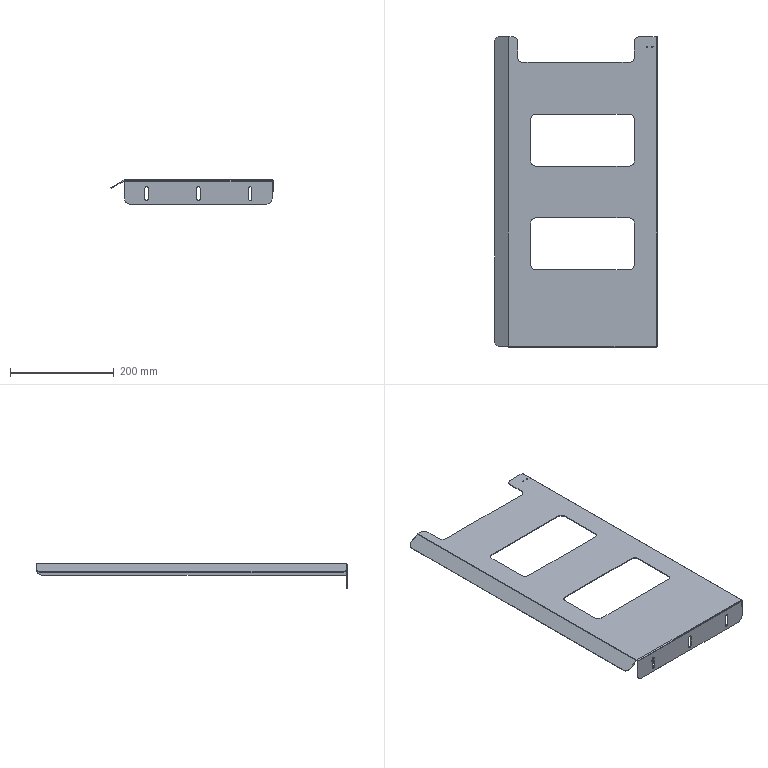Part | STEP file | PN_0024(Default) | 1 solid | 83 faces | box 313.731 x 599.997 x 46.5 mm | volume 244261 mm3 | plane 43 | cylinder 40 | commonest cylinder face diameters 20 x17 6.5 x9 2.5 x4 4.2 x4 1.473 x3 4.473 x3